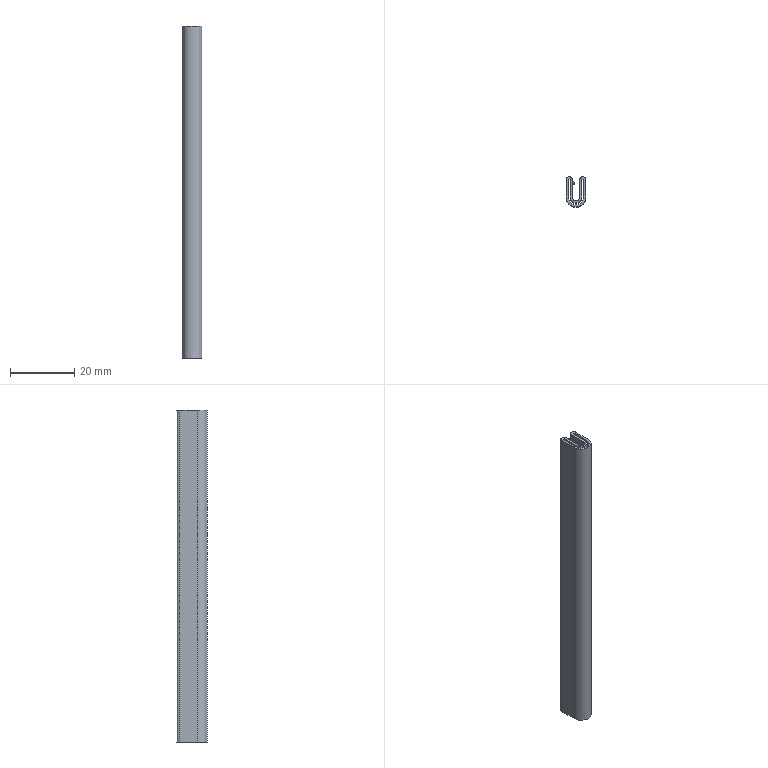Part | STEP file | TRAT2_4_B_3L1_TRAT2.4-B-3-L1 | 1 solid | 22 faces | box 6.2 x 9.5 x 103.6 mm | volume 2671 mm3 | plane 15 | cylinder 7 | commonest cylinder face diameters 1.9 x2 0.4 x1 2.4 x1 3.692 x1 4.933 x1 6.2 x1
STEP:
#1=CARTESIAN_POINT('',(1.9,8.55,103.6));
#2=VERTEX_POINT('',#1);
#3=CARTESIAN_POINT('',(0.,8.55,103.6));
#4=VERTEX_POINT('',#3);
#5=CARTESIAN_POINT('',(0.95,8.55,103.6));
#6=DIRECTION('',(0.,0.,1.));
#7=DIRECTION('',(1.,0.,0.));
#8=AXIS2_PLACEMENT_3D('',#5,#6,#7);
#9=CIRCLE('',#8,0.95);
#10=EDGE_CURVE('',#2,#4,#9,.T.);
#11=ORIENTED_EDGE('',*,*,#10,.T.);
#12=CARTESIAN_POINT('',(0.,3.1,103.6));
#13=VERTEX_POINT('',#12);
#14=CARTESIAN_POINT('',(0.,8.55,103.6));
#15=DIRECTION('',(0.,-1.,0.));
#16=VECTOR('',#15,1000.);
#17=LINE('',#14,#16);
#18=EDGE_CURVE('',#4,#13,#17,.T.);
#19=ORIENTED_EDGE('',*,*,#18,.T.);
#20=CARTESIAN_POINT('',(6.2,3.1,103.6));
#21=VERTEX_POINT('',#20);
#22=CARTESIAN_POINT('',(3.1,3.1,103.6));
#23=DIRECTION('',(0.,0.,1.));
#24=DIRECTION('',(1.,0.,0.));
#25=AXIS2_PLACEMENT_3D('',#22,#23,#24);
#26=CIRCLE('',#25,3.1);
#27=EDGE_CURVE('',#13,#21,#26,.T.);
#28=ORIENTED_EDGE('',*,*,#27,.T.);
#29=CARTESIAN_POINT('',(6.2,8.55,103.6));
#30=VERTEX_POINT('',#29);
#31=CARTESIAN_POINT('',(6.2,3.1,103.6));
#32=DIRECTION('',(0.,1.,0.));
#33=VECTOR('',#32,1000.);
#34=LINE('',#31,#33);
#35=EDGE_CURVE('',#21,#30,#34,.T.);
#36=ORIENTED_EDGE('',*,*,#35,.T.);
#37=CARTESIAN_POINT('',(4.3,8.55,103.6));
#38=VERTEX_POINT('',#37);
#39=CARTESIAN_POINT('',(5.25,8.55,103.6));
#40=DIRECTION('',(0.,0.,1.));
#41=DIRECTION('',(1.,0.,0.));
#42=AXIS2_PLACEMENT_3D('',#39,#40,#41);
#43=CIRCLE('',#42,0.95);
#44=EDGE_CURVE('',#30,#38,#43,.T.);
#45=ORIENTED_EDGE('',*,*,#44,.T.);
#46=CARTESIAN_POINT('',(4.3,3.1,103.6));
#47=VERTEX_POINT('',#46);
#48=CARTESIAN_POINT('',(4.3,8.55,103.6));
#49=DIRECTION('',(0.,-1.,0.));
#50=VECTOR('',#49,1000.);
#51=LINE('',#48,#50);
#52=EDGE_CURVE('',#38,#47,#51,.T.);
#53=ORIENTED_EDGE('',*,*,#52,.T.);
#54=CARTESIAN_POINT('',(1.9,3.1,103.6));
#55=VERTEX_POINT('',#54);
#56=CARTESIAN_POINT('',(3.1,3.1,103.6));
#57=DIRECTION('',(0.,0.,-1.));
#58=DIRECTION('',(-1.,0.,0.));
#59=AXIS2_PLACEMENT_3D('',#56,#57,#58);
#60=CIRCLE('',#59,1.2);
#61=EDGE_CURVE('',#47,#55,#60,.T.);
#62=ORIENTED_EDGE('',*,*,#61,.T.);
#63=CARTESIAN_POINT('',(1.9,7.6,103.6));
#64=VERTEX_POINT('',#63);
#65=CARTESIAN_POINT('',(1.9,3.1,103.6));
#66=DIRECTION('',(0.,1.,0.));
#67=VECTOR('',#66,1000.);
#68=LINE('',#65,#67);
#69=EDGE_CURVE('',#55,#64,#68,.T.);
#70=ORIENTED_EDGE('',*,*,#69,.T.);
#71=CARTESIAN_POINT('',(2.472,7.27,103.6));
#72=VERTEX_POINT('',#71);
#73=CARTESIAN_POINT('',(1.9,7.6,103.6));
#74=DIRECTION('',(0.866,-0.5,0.));
#75=VECTOR('',#74,1000.);
#76=LINE('',#73,#75);
#77=EDGE_CURVE('',#64,#72,#76,.T.);
#78=ORIENTED_EDGE('',*,*,#77,.T.);
#79=CARTESIAN_POINT('',(2.672,7.616,103.6));
#80=VERTEX_POINT('',#79);
#81=CARTESIAN_POINT('',(2.572,7.443,103.6));
#82=DIRECTION('',(0.,0.,1.));
#83=DIRECTION('',(1.,0.,0.));
#84=AXIS2_PLACEMENT_3D('',#81,#82,#83);
#85=CIRCLE('',#84,0.2);
#86=EDGE_CURVE('',#72,#80,#85,.T.);
#87=ORIENTED_EDGE('',*,*,#86,.T.);
#88=CARTESIAN_POINT('',(1.9,8.062,103.6));
#89=VERTEX_POINT('',#88);
#90=CARTESIAN_POINT('',(2.672,7.616,103.6));
#91=DIRECTION('',(-0.866,0.5,0.));
#92=VECTOR('',#91,1000.);
#93=LINE('',#90,#92);
#94=EDGE_CURVE('',#80,#89,#93,.T.);
#95=ORIENTED_EDGE('',*,*,#94,.T.);
#96=CARTESIAN_POINT('',(1.9,8.062,103.6));
#97=DIRECTION('',(0.,1.,0.));
#98=VECTOR('',#97,1000.);
#99=LINE('',#96,#98);
#100=EDGE_CURVE('',#89,#2,#99,.T.);
#101=ORIENTED_EDGE('',*,*,#100,.T.);
#102=EDGE_LOOP('',(#11,#19,#28,#36,#45,#53,#62,#70,#78,#87,#95,#101));
#103=FACE_OUTER_BOUND('',#102,.T.);
#104=CARTESIAN_POINT('',(0.6333,8.55,103.6));
#105=VERTEX_POINT('',#104);
#106=CARTESIAN_POINT('',(0.6333,3.1,103.6));
#107=VERTEX_POINT('',#106);
#108=CARTESIAN_POINT('',(0.6333,8.55,103.6));
#109=DIRECTION('',(0.,-1.,0.));
#110=VECTOR('',#109,1000.);
#111=LINE('',#108,#110);
#112=EDGE_CURVE('',#105,#107,#111,.T.);
#113=ORIENTED_EDGE('',*,*,#112,.F.);
#114=CARTESIAN_POINT('',(1.254,8.55,103.6));
#115=VERTEX_POINT('',#114);
#116=CARTESIAN_POINT('',(1.254,8.55,103.6));
#117=DIRECTION('',(-1.,0.,0.));
#118=VECTOR('',#117,1000.);
#119=LINE('',#116,#118);
#120=EDGE_CURVE('',#115,#105,#119,.T.);
#121=ORIENTED_EDGE('',*,*,#120,.F.);
#122=CARTESIAN_POINT('',(1.254,3.1,103.6));
#123=VERTEX_POINT('',#122);
#124=CARTESIAN_POINT('',(1.254,3.1,103.6));
#125=DIRECTION('',(0.,1.,0.));
#126=VECTOR('',#125,1000.);
#127=LINE('',#124,#126);
#128=EDGE_CURVE('',#123,#115,#127,.T.);
#129=ORIENTED_EDGE('',*,*,#128,.F.);
#130=CARTESIAN_POINT('',(4.946,3.1,103.6));
#131=VERTEX_POINT('',#130);
#132=CARTESIAN_POINT('',(3.1,3.1,103.6));
#133=DIRECTION('',(0.,0.,-1.));
#134=DIRECTION('',(-1.,0.,0.));
#135=AXIS2_PLACEMENT_3D('',#132,#133,#134);
#136=CIRCLE('',#135,1.846);
#137=EDGE_CURVE('',#131,#123,#136,.T.);
#138=ORIENTED_EDGE('',*,*,#137,.F.);
#139=CARTESIAN_POINT('',(4.946,8.55,103.6));
#140=VERTEX_POINT('',#139);
#141=CARTESIAN_POINT('',(4.946,8.55,103.6));
#142=DIRECTION('',(0.,-1.,0.));
#143=VECTOR('',#142,1000.);
#144=LINE('',#141,#143);
#145=EDGE_CURVE('',#140,#131,#144,.T.);
#146=ORIENTED_EDGE('',*,*,#145,.F.);
#147=CARTESIAN_POINT('',(5.567,8.55,103.6));
#148=VERTEX_POINT('',#147);
#149=CARTESIAN_POINT('',(5.567,8.55,103.6));
#150=DIRECTION('',(-1.,0.,0.));
#151=VECTOR('',#150,1000.);
#152=LINE('',#149,#151);
#153=EDGE_CURVE('',#148,#140,#152,.T.);
#154=ORIENTED_EDGE('',*,*,#153,.F.);
#155=CARTESIAN_POINT('',(5.567,3.1,103.6));
#156=VERTEX_POINT('',#155);
#157=CARTESIAN_POINT('',(5.567,3.1,103.6));
#158=DIRECTION('',(0.,1.,0.));
#159=VECTOR('',#158,1000.);
#160=LINE('',#157,#159);
#161=EDGE_CURVE('',#156,#148,#160,.T.);
#162=ORIENTED_EDGE('',*,*,#161,.F.);
#163=CARTESIAN_POINT('',(3.1,3.1,103.6));
#164=DIRECTION('',(0.,0.,1.));
#165=DIRECTION('',(1.,0.,0.));
#166=AXIS2_PLACEMENT_3D('',#163,#164,#165);
#167=CIRCLE('',#166,2.467);
#168=EDGE_CURVE('',#107,#156,#167,.T.);
#169=ORIENTED_EDGE('',*,*,#168,.F.);
#170=EDGE_LOOP('',(#113,#121,#129,#138,#146,#154,#162,#169));
#171=FACE_BOUND('',#170,.T.);
#172=CARTESIAN_POINT('',(0.95,8.55,103.6));
#173=DIRECTION('',(0.,0.,1.));
#174=DIRECTION('',(1.,0.,0.));
#175=AXIS2_PLACEMENT_3D('',#172,#173,#174);
#176=PLANE('',#175);
#177=ADVANCED_FACE('',(#103,#171),#176,.T.);
#178=CARTESIAN_POINT('',(1.9,8.55,0.));
#179=VERTEX_POINT('',#178);
#180=CARTESIAN_POINT('',(0.,8.55,0.));
#181=VERTEX_POINT('',#180);
#182=CARTESIAN_POINT('',(0.95,8.55,0.));
#183=DIRECTION('',(0.,0.,1.));
#184=DIRECTION('',(1.,0.,0.));
#185=AXIS2_PLACEMENT_3D('',#182,#183,#184);
#186=CIRCLE('',#185,0.95);
#187=EDGE_CURVE('',#179,#181,#186,.T.);
#188=ORIENTED_EDGE('',*,*,#187,.F.);
#189=CARTESIAN_POINT('',(1.9,8.062,0.));
#190=VERTEX_POINT('',#189);
#191=CARTESIAN_POINT('',(1.9,8.062,0.));
#192=DIRECTION('',(0.,1.,0.));
#193=VECTOR('',#192,1000.);
#194=LINE('',#191,#193);
#195=EDGE_CURVE('',#190,#179,#194,.T.);
#196=ORIENTED_EDGE('',*,*,#195,.F.);
#197=CARTESIAN_POINT('',(2.672,7.616,0.));
#198=VERTEX_POINT('',#197);
#199=CARTESIAN_POINT('',(2.672,7.616,0.));
#200=DIRECTION('',(-0.866,0.5,0.));
#201=VECTOR('',#200,1000.);
#202=LINE('',#199,#201);
#203=EDGE_CURVE('',#198,#190,#202,.T.);
#204=ORIENTED_EDGE('',*,*,#203,.F.);
#205=CARTESIAN_POINT('',(2.472,7.27,0.));
#206=VERTEX_POINT('',#205);
#207=CARTESIAN_POINT('',(2.572,7.443,0.));
#208=DIRECTION('',(0.,0.,1.));
#209=DIRECTION('',(1.,0.,0.));
#210=AXIS2_PLACEMENT_3D('',#207,#208,#209);
#211=CIRCLE('',#210,0.2);
#212=EDGE_CURVE('',#206,#198,#211,.T.);
#213=ORIENTED_EDGE('',*,*,#212,.F.);
#214=CARTESIAN_POINT('',(1.9,7.6,0.));
#215=VERTEX_POINT('',#214);
#216=CARTESIAN_POINT('',(1.9,7.6,0.));
#217=DIRECTION('',(0.866,-0.5,0.));
#218=VECTOR('',#217,1000.);
#219=LINE('',#216,#218);
#220=EDGE_CURVE('',#215,#206,#219,.T.);
#221=ORIENTED_EDGE('',*,*,#220,.F.);
#222=CARTESIAN_POINT('',(1.9,3.1,0.));
#223=VERTEX_POINT('',#222);
#224=CARTESIAN_POINT('',(1.9,3.1,0.));
#225=DIRECTION('',(0.,1.,0.));
#226=VECTOR('',#225,1000.);
#227=LINE('',#224,#226);
#228=EDGE_CURVE('',#223,#215,#227,.T.);
#229=ORIENTED_EDGE('',*,*,#228,.F.);
#230=CARTESIAN_POINT('',(4.3,3.1,0.));
#231=VERTEX_POINT('',#230);
#232=CARTESIAN_POINT('',(3.1,3.1,0.));
#233=DIRECTION('',(0.,0.,-1.));
#234=DIRECTION('',(-1.,0.,0.));
#235=AXIS2_PLACEMENT_3D('',#232,#233,#234);
#236=CIRCLE('',#235,1.2);
#237=EDGE_CURVE('',#231,#223,#236,.T.);
#238=ORIENTED_EDGE('',*,*,#237,.F.);
#239=CARTESIAN_POINT('',(4.3,8.55,0.));
#240=VERTEX_POINT('',#239);
#241=CARTESIAN_POINT('',(4.3,8.55,0.));
#242=DIRECTION('',(0.,-1.,0.));
#243=VECTOR('',#242,1000.);
#244=LINE('',#241,#243);
#245=EDGE_CURVE('',#240,#231,#244,.T.);
#246=ORIENTED_EDGE('',*,*,#245,.F.);
#247=CARTESIAN_POINT('',(6.2,8.55,0.));
#248=VERTEX_POINT('',#247);
#249=CARTESIAN_POINT('',(5.25,8.55,0.));
#250=DIRECTION('',(0.,0.,1.));
#251=DIRECTION('',(1.,0.,0.));
#252=AXIS2_PLACEMENT_3D('',#249,#250,#251);
#253=CIRCLE('',#252,0.95);
#254=EDGE_CURVE('',#248,#240,#253,.T.);
#255=ORIENTED_EDGE('',*,*,#254,.F.);
#256=CARTESIAN_POINT('',(6.2,3.1,0.));
#257=VERTEX_POINT('',#256);
#258=CARTESIAN_POINT('',(6.2,3.1,0.));
#259=DIRECTION('',(0.,1.,0.));
#260=VECTOR('',#259,1000.);
#261=LINE('',#258,#260);
#262=EDGE_CURVE('',#257,#248,#261,.T.);
#263=ORIENTED_EDGE('',*,*,#262,.F.);
#264=CARTESIAN_POINT('',(0.,3.1,0.));
#265=VERTEX_POINT('',#264);
#266=CARTESIAN_POINT('',(3.1,3.1,0.));
#267=DIRECTION('',(0.,0.,1.));
#268=DIRECTION('',(1.,0.,0.));
#269=AXIS2_PLACEMENT_3D('',#266,#267,#268);
#270=CIRCLE('',#269,3.1);
#271=EDGE_CURVE('',#265,#257,#270,.T.);
#272=ORIENTED_EDGE('',*,*,#271,.F.);
#273=CARTESIAN_POINT('',(0.,8.55,0.));
#274=DIRECTION('',(0.,-1.,0.));
#275=VECTOR('',#274,1000.);
#276=LINE('',#273,#275);
#277=EDGE_CURVE('',#181,#265,#276,.T.);
#278=ORIENTED_EDGE('',*,*,#277,.F.);
#279=EDGE_LOOP('',(#188,#196,#204,#213,#221,#229,#238,#246,#255,#263,#272,#278));
#280=FACE_OUTER_BOUND('',#279,.T.);
#281=CARTESIAN_POINT('',(1.254,8.55,0.));
#282=VERTEX_POINT('',#281);
#283=CARTESIAN_POINT('',(0.6333,8.55,0.));
#284=VERTEX_POINT('',#283);
#285=CARTESIAN_POINT('',(1.254,8.55,0.));
#286=DIRECTION('',(-1.,0.,0.));
#287=VECTOR('',#286,1000.);
#288=LINE('',#285,#287);
#289=EDGE_CURVE('',#282,#284,#288,.T.);
#290=ORIENTED_EDGE('',*,*,#289,.T.);
#291=CARTESIAN_POINT('',(0.6333,3.1,0.));
#292=VERTEX_POINT('',#291);
#293=CARTESIAN_POINT('',(0.6333,8.55,0.));
#294=DIRECTION('',(0.,-1.,0.));
#295=VECTOR('',#294,1000.);
#296=LINE('',#293,#295);
#297=EDGE_CURVE('',#284,#292,#296,.T.);
#298=ORIENTED_EDGE('',*,*,#297,.T.);
#299=CARTESIAN_POINT('',(5.567,3.1,0.));
#300=VERTEX_POINT('',#299);
#301=CARTESIAN_POINT('',(3.1,3.1,0.));
#302=DIRECTION('',(0.,0.,1.));
#303=DIRECTION('',(1.,0.,0.));
#304=AXIS2_PLACEMENT_3D('',#301,#302,#303);
#305=CIRCLE('',#304,2.467);
#306=EDGE_CURVE('',#292,#300,#305,.T.);
#307=ORIENTED_EDGE('',*,*,#306,.T.);
#308=CARTESIAN_POINT('',(5.567,8.55,0.));
#309=VERTEX_POINT('',#308);
#310=CARTESIAN_POINT('',(5.567,3.1,0.));
#311=DIRECTION('',(0.,1.,0.));
#312=VECTOR('',#311,1000.);
#313=LINE('',#310,#312);
#314=EDGE_CURVE('',#300,#309,#313,.T.);
#315=ORIENTED_EDGE('',*,*,#314,.T.);
#316=CARTESIAN_POINT('',(4.946,8.55,0.));
#317=VERTEX_POINT('',#316);
#318=CARTESIAN_POINT('',(5.567,8.55,0.));
#319=DIRECTION('',(-1.,0.,0.));
#320=VECTOR('',#319,1000.);
#321=LINE('',#318,#320);
#322=EDGE_CURVE('',#309,#317,#321,.T.);
#323=ORIENTED_EDGE('',*,*,#322,.T.);
#324=CARTESIAN_POINT('',(4.946,3.1,0.));
#325=VERTEX_POINT('',#324);
#326=CARTESIAN_POINT('',(4.946,8.55,0.));
#327=DIRECTION('',(0.,-1.,0.));
#328=VECTOR('',#327,1000.);
#329=LINE('',#326,#328);
#330=EDGE_CURVE('',#317,#325,#329,.T.);
#331=ORIENTED_EDGE('',*,*,#330,.T.);
#332=CARTESIAN_POINT('',(1.254,3.1,0.));
#333=VERTEX_POINT('',#332);
#334=CARTESIAN_POINT('',(3.1,3.1,0.));
#335=DIRECTION('',(0.,0.,-1.));
#336=DIRECTION('',(-1.,0.,0.));
#337=AXIS2_PLACEMENT_3D('',#334,#335,#336);
#338=CIRCLE('',#337,1.846);
#339=EDGE_CURVE('',#325,#333,#338,.T.);
#340=ORIENTED_EDGE('',*,*,#339,.T.);
#341=CARTESIAN_POINT('',(1.254,3.1,0.));
#342=DIRECTION('',(0.,1.,0.));
#343=VECTOR('',#342,1000.);
#344=LINE('',#341,#343);
#345=EDGE_CURVE('',#333,#282,#344,.T.);
#346=ORIENTED_EDGE('',*,*,#345,.T.);
#347=EDGE_LOOP('',(#290,#298,#307,#315,#323,#331,#340,#346));
#348=FACE_BOUND('',#347,.T.);
#349=CARTESIAN_POINT('',(0.95,8.55,0.));
#350=DIRECTION('',(0.,0.,1.));
#351=DIRECTION('',(1.,0.,0.));
#352=AXIS2_PLACEMENT_3D('',#349,#350,#351);
#353=PLANE('',#352);
#354=ADVANCED_FACE('',(#280,#348),#353,.F.);
#355=ORIENTED_EDGE('',*,*,#187,.T.);
#356=CARTESIAN_POINT('',(0.,8.55,103.6));
#357=DIRECTION('',(0.,0.,-1.));
#358=VECTOR('',#357,1000.);
#359=LINE('',#356,#358);
#360=EDGE_CURVE('',#4,#181,#359,.T.);
#361=ORIENTED_EDGE('',*,*,#360,.F.);
#362=ORIENTED_EDGE('',*,*,#10,.F.);
#363=CARTESIAN_POINT('',(1.9,8.55,103.6));
#364=DIRECTION('',(0.,0.,-1.));
#365=VECTOR('',#364,1000.);
#366=LINE('',#363,#365);
#367=EDGE_CURVE('',#2,#179,#366,.T.);
#368=ORIENTED_EDGE('',*,*,#367,.T.);
#369=EDGE_LOOP('',(#355,#361,#362,#368));
#370=FACE_OUTER_BOUND('',#369,.T.);
#371=CARTESIAN_POINT('',(0.95,8.55,103.6));
#372=DIRECTION('',(0.,0.,-1.));
#373=DIRECTION('',(-1.,0.,0.));
#374=AXIS2_PLACEMENT_3D('',#371,#372,#373);
#375=CYLINDRICAL_SURFACE('',#374,0.95);
#376=ADVANCED_FACE('',(#370),#375,.T.);
#377=ORIENTED_EDGE('',*,*,#277,.T.);
#378=CARTESIAN_POINT('',(0.,3.1,103.6));
#379=DIRECTION('',(0.,0.,-1.));
#380=VECTOR('',#379,1000.);
#381=LINE('',#378,#380);
#382=EDGE_CURVE('',#13,#265,#381,.T.);
#383=ORIENTED_EDGE('',*,*,#382,.F.);
#384=ORIENTED_EDGE('',*,*,#18,.F.);
#385=ORIENTED_EDGE('',*,*,#360,.T.);
#386=EDGE_LOOP('',(#377,#383,#384,#385));
#387=FACE_OUTER_BOUND('',#386,.T.);
#388=CARTESIAN_POINT('',(0.,8.55,103.6));
#389=DIRECTION('',(1.,0.,0.));
#390=DIRECTION('',(0.,0.,-1.));
#391=AXIS2_PLACEMENT_3D('',#388,#389,#390);
#392=PLANE('',#391);
#393=ADVANCED_FACE('',(#387),#392,.F.);
#394=ORIENTED_EDGE('',*,*,#271,.T.);
#395=CARTESIAN_POINT('',(6.2,3.1,103.6));
#396=DIRECTION('',(0.,0.,-1.));
#397=VECTOR('',#396,1000.);
#398=LINE('',#395,#397);
#399=EDGE_CURVE('',#21,#257,#398,.T.);
#400=ORIENTED_EDGE('',*,*,#399,.F.);
#401=ORIENTED_EDGE('',*,*,#27,.F.);
#402=ORIENTED_EDGE('',*,*,#382,.T.);
#403=EDGE_LOOP('',(#394,#400,#401,#402));
#404=FACE_OUTER_BOUND('',#403,.T.);
#405=CARTESIAN_POINT('',(3.1,3.1,103.6));
#406=DIRECTION('',(0.,0.,-1.));
#407=DIRECTION('',(-1.,0.,0.));
#408=AXIS2_PLACEMENT_3D('',#405,#406,#407);
#409=CYLINDRICAL_SURFACE('',#408,3.1);
#410=ADVANCED_FACE('',(#404),#409,.T.);
#411=ORIENTED_EDGE('',*,*,#262,.T.);
#412=CARTESIAN_POINT('',(6.2,8.55,103.6));
#413=DIRECTION('',(0.,0.,-1.));
#414=VECTOR('',#413,1000.);
#415=LINE('',#412,#414);
#416=EDGE_CURVE('',#30,#248,#415,.T.);
#417=ORIENTED_EDGE('',*,*,#416,.F.);
#418=ORIENTED_EDGE('',*,*,#35,.F.);
#419=ORIENTED_EDGE('',*,*,#399,.T.);
#420=EDGE_LOOP('',(#411,#417,#418,#419));
#421=FACE_OUTER_BOUND('',#420,.T.);
#422=CARTESIAN_POINT('',(6.2,3.1,103.6));
#423=DIRECTION('',(-1.,0.,0.));
#424=DIRECTION('',(0.,0.,1.));
#425=AXIS2_PLACEMENT_3D('',#422,#423,#424);
#426=PLANE('',#425);
#427=ADVANCED_FACE('',(#421),#426,.F.);
#428=ORIENTED_EDGE('',*,*,#254,.T.);
#429=CARTESIAN_POINT('',(4.3,8.55,103.6));
#430=DIRECTION('',(0.,0.,-1.));
#431=VECTOR('',#430,1000.);
#432=LINE('',#429,#431);
#433=EDGE_CURVE('',#38,#240,#432,.T.);
#434=ORIENTED_EDGE('',*,*,#433,.F.);
#435=ORIENTED_EDGE('',*,*,#44,.F.);
#436=ORIENTED_EDGE('',*,*,#416,.T.);
#437=EDGE_LOOP('',(#428,#434,#435,#436));
#438=FACE_OUTER_BOUND('',#437,.T.);
#439=CARTESIAN_POINT('',(5.25,8.55,103.6));
#440=DIRECTION('',(0.,0.,-1.));
#441=DIRECTION('',(-1.,0.,0.));
#442=AXIS2_PLACEMENT_3D('',#439,#440,#441);
#443=CYLINDRICAL_SURFACE('',#442,0.95);
#444=ADVANCED_FACE('',(#438),#443,.T.);
#445=ORIENTED_EDGE('',*,*,#245,.T.);
#446=CARTESIAN_POINT('',(4.3,3.1,103.6));
#447=DIRECTION('',(0.,0.,-1.));
#448=VECTOR('',#447,1000.);
#449=LINE('',#446,#448);
#450=EDGE_CURVE('',#47,#231,#449,.T.);
#451=ORIENTED_EDGE('',*,*,#450,.F.);
#452=ORIENTED_EDGE('',*,*,#52,.F.);
#453=ORIENTED_EDGE('',*,*,#433,.T.);
#454=EDGE_LOOP('',(#445,#451,#452,#453));
#455=FACE_OUTER_BOUND('',#454,.T.);
#456=CARTESIAN_POINT('',(4.3,8.55,103.6));
#457=DIRECTION('',(1.,0.,0.));
#458=DIRECTION('',(0.,1.,0.));
#459=AXIS2_PLACEMENT_3D('',#456,#457,#458);
#460=PLANE('',#459);
#461=ADVANCED_FACE('',(#455),#460,.F.);
#462=ORIENTED_EDGE('',*,*,#237,.T.);
#463=CARTESIAN_POINT('',(1.9,3.1,103.6));
#464=DIRECTION('',(0.,0.,-1.));
#465=VECTOR('',#464,1000.);
#466=LINE('',#463,#465);
#467=EDGE_CURVE('',#55,#223,#466,.T.);
#468=ORIENTED_EDGE('',*,*,#467,.F.);
#469=ORIENTED_EDGE('',*,*,#61,.F.);
#470=ORIENTED_EDGE('',*,*,#450,.T.);
#471=EDGE_LOOP('',(#462,#468,#469,#470));
#472=FACE_OUTER_BOUND('',#471,.T.);
#473=CARTESIAN_POINT('',(3.1,3.1,103.6));
#474=DIRECTION('',(0.,0.,-1.));
#475=DIRECTION('',(-1.,0.,0.));
#476=AXIS2_PLACEMENT_3D('',#473,#474,#475);
#477=CYLINDRICAL_SURFACE('',#476,1.2);
#478=ADVANCED_FACE('',(#472),#477,.F.);
#479=ORIENTED_EDGE('',*,*,#228,.T.);
#480=CARTESIAN_POINT('',(1.9,7.6,103.6));
#481=DIRECTION('',(0.,0.,-1.));
#482=VECTOR('',#481,1000.);
#483=LINE('',#480,#482);
#484=EDGE_CURVE('',#64,#215,#483,.T.);
#485=ORIENTED_EDGE('',*,*,#484,.F.);
#486=ORIENTED_EDGE('',*,*,#69,.F.);
#487=ORIENTED_EDGE('',*,*,#467,.T.);
#488=EDGE_LOOP('',(#479,#485,#486,#487));
#489=FACE_OUTER_BOUND('',#488,.T.);
#490=CARTESIAN_POINT('',(1.9,3.1,103.6));
#491=DIRECTION('',(-1.,0.,0.));
#492=DIRECTION('',(0.,-1.,0.));
#493=AXIS2_PLACEMENT_3D('',#490,#491,#492);
#494=PLANE('',#493);
#495=ADVANCED_FACE('',(#489),#494,.F.);
#496=ORIENTED_EDGE('',*,*,#220,.T.);
#497=CARTESIAN_POINT('',(2.472,7.27,103.6));
#498=DIRECTION('',(0.,0.,-1.));
#499=VECTOR('',#498,1000.);
#500=LINE('',#497,#499);
#501=EDGE_CURVE('',#72,#206,#500,.T.);
#502=ORIENTED_EDGE('',*,*,#501,.F.);
#503=ORIENTED_EDGE('',*,*,#77,.F.);
#504=ORIENTED_EDGE('',*,*,#484,.T.);
#505=EDGE_LOOP('',(#496,#502,#503,#504));
#506=FACE_OUTER_BOUND('',#505,.T.);
#507=CARTESIAN_POINT('',(1.9,7.6,103.6));
#508=DIRECTION('',(0.5,0.866,0.));
#509=DIRECTION('',(-0.866,0.5,0.));
#510=AXIS2_PLACEMENT_3D('',#507,#508,#509);
#511=PLANE('',#510);
#512=ADVANCED_FACE('',(#506),#511,.F.);
#513=ORIENTED_EDGE('',*,*,#212,.T.);
#514=CARTESIAN_POINT('',(2.672,7.616,103.6));
#515=DIRECTION('',(0.,0.,-1.));
#516=VECTOR('',#515,1000.);
#517=LINE('',#514,#516);
#518=EDGE_CURVE('',#80,#198,#517,.T.);
#519=ORIENTED_EDGE('',*,*,#518,.F.);
#520=ORIENTED_EDGE('',*,*,#86,.F.);
#521=ORIENTED_EDGE('',*,*,#501,.T.);
#522=EDGE_LOOP('',(#513,#519,#520,#521));
#523=FACE_OUTER_BOUND('',#522,.T.);
#524=CARTESIAN_POINT('',(2.572,7.443,103.6));
#525=DIRECTION('',(0.,0.,-1.));
#526=DIRECTION('',(-1.,0.,0.));
#527=AXIS2_PLACEMENT_3D('',#524,#525,#526);
#528=CYLINDRICAL_SURFACE('',#527,0.2);
#529=ADVANCED_FACE('',(#523),#528,.T.);
#530=ORIENTED_EDGE('',*,*,#203,.T.);
#531=CARTESIAN_POINT('',(1.9,8.062,103.6));
#532=DIRECTION('',(0.,0.,-1.));
#533=VECTOR('',#532,1000.);
#534=LINE('',#531,#533);
#535=EDGE_CURVE('',#89,#190,#534,.T.);
#536=ORIENTED_EDGE('',*,*,#535,.F.);
#537=ORIENTED_EDGE('',*,*,#94,.F.);
#538=ORIENTED_EDGE('',*,*,#518,.T.);
#539=EDGE_LOOP('',(#530,#536,#537,#538));
#540=FACE_OUTER_BOUND('',#539,.T.);
#541=CARTESIAN_POINT('',(2.672,7.616,103.6));
#542=DIRECTION('',(-0.5,-0.866,0.));
#543=DIRECTION('',(0.866,-0.5,0.));
#544=AXIS2_PLACEMENT_3D('',#541,#542,#543);
#545=PLANE('',#544);
#546=ADVANCED_FACE('',(#540),#545,.F.);
#547=ORIENTED_EDGE('',*,*,#195,.T.);
#548=ORIENTED_EDGE('',*,*,#367,.F.);
#549=ORIENTED_EDGE('',*,*,#100,.F.);
#550=ORIENTED_EDGE('',*,*,#535,.T.);
#551=EDGE_LOOP('',(#547,#548,#549,#550));
#552=FACE_OUTER_BOUND('',#551,.T.);
#553=CARTESIAN_POINT('',(1.9,8.062,103.6));
#554=DIRECTION('',(-1.,0.,0.));
#555=DIRECTION('',(0.,0.,1.));
#556=AXIS2_PLACEMENT_3D('',#553,#554,#555);
#557=PLANE('',#556);
#558=ADVANCED_FACE('',(#552),#557,.F.);
#559=ORIENTED_EDGE('',*,*,#289,.F.);
#560=CARTESIAN_POINT('',(1.254,8.55,103.6));
#561=DIRECTION('',(0.,0.,-1.));
#562=VECTOR('',#561,1000.);
#563=LINE('',#560,#562);
#564=EDGE_CURVE('',#115,#282,#563,.T.);
#565=ORIENTED_EDGE('',*,*,#564,.F.);
#566=ORIENTED_EDGE('',*,*,#120,.T.);
#567=CARTESIAN_POINT('',(0.6333,8.55,103.6));
#568=DIRECTION('',(0.,0.,-1.));
#569=VECTOR('',#568,1000.);
#570=LINE('',#567,#569);
#571=EDGE_CURVE('',#105,#284,#570,.T.);
#572=ORIENTED_EDGE('',*,*,#571,.T.);
#573=EDGE_LOOP('',(#559,#565,#566,#572));
#574=FACE_OUTER_BOUND('',#573,.T.);
#575=CARTESIAN_POINT('',(1.254,8.55,103.6));
#576=DIRECTION('',(0.,-1.,0.));
#577=DIRECTION('',(0.,0.,-1.));
#578=AXIS2_PLACEMENT_3D('',#575,#576,#577);
#579=PLANE('',#578);
#580=ADVANCED_FACE('',(#574),#579,.T.);
#581=ORIENTED_EDGE('',*,*,#297,.F.);
#582=ORIENTED_EDGE('',*,*,#571,.F.);
#583=ORIENTED_EDGE('',*,*,#112,.T.);
#584=CARTESIAN_POINT('',(0.6333,3.1,103.6));
#585=DIRECTION('',(0.,0.,-1.));
#586=VECTOR('',#585,1000.);
#587=LINE('',#584,#586);
#588=EDGE_CURVE('',#107,#292,#587,.T.);
#589=ORIENTED_EDGE('',*,*,#588,.T.);
#590=EDGE_LOOP('',(#581,#582,#583,#589));
#591=FACE_OUTER_BOUND('',#590,.T.);
#592=CARTESIAN_POINT('',(0.6333,8.55,103.6));
#593=DIRECTION('',(1.,0.,0.));
#594=DIRECTION('',(0.,1.,0.));
#595=AXIS2_PLACEMENT_3D('',#592,#593,#594);
#596=PLANE('',#595);
#597=ADVANCED_FACE('',(#591),#596,.T.);
#598=ORIENTED_EDGE('',*,*,#306,.F.);
#599=ORIENTED_EDGE('',*,*,#588,.F.);
#600=ORIENTED_EDGE('',*,*,#168,.T.);
#601=CARTESIAN_POINT('',(5.567,3.1,103.6));
#602=DIRECTION('',(0.,0.,-1.));
#603=VECTOR('',#602,1000.);
#604=LINE('',#601,#603);
#605=EDGE_CURVE('',#156,#300,#604,.T.);
#606=ORIENTED_EDGE('',*,*,#605,.T.);
#607=EDGE_LOOP('',(#598,#599,#600,#606));
#608=FACE_OUTER_BOUND('',#607,.T.);
#609=CARTESIAN_POINT('',(3.1,3.1,103.6));
#610=DIRECTION('',(0.,0.,-1.));
#611=DIRECTION('',(-1.,0.,0.));
#612=AXIS2_PLACEMENT_3D('',#609,#610,#611);
#613=CYLINDRICAL_SURFACE('',#612,2.467);
#614=ADVANCED_FACE('',(#608),#613,.F.);
#615=ORIENTED_EDGE('',*,*,#314,.F.);
#616=ORIENTED_EDGE('',*,*,#605,.F.);
#617=ORIENTED_EDGE('',*,*,#161,.T.);
#618=CARTESIAN_POINT('',(5.567,8.55,103.6));
#619=DIRECTION('',(0.,0.,-1.));
#620=VECTOR('',#619,1000.);
#621=LINE('',#618,#620);
#622=EDGE_CURVE('',#148,#309,#621,.T.);
#623=ORIENTED_EDGE('',*,*,#622,.T.);
#624=EDGE_LOOP('',(#615,#616,#617,#623));
#625=FACE_OUTER_BOUND('',#624,.T.);
#626=CARTESIAN_POINT('',(5.567,3.1,103.6));
#627=DIRECTION('',(-1.,0.,0.));
#628=DIRECTION('',(0.,-1.,0.));
#629=AXIS2_PLACEMENT_3D('',#626,#627,#628);
#630=PLANE('',#629);
#631=ADVANCED_FACE('',(#625),#630,.T.);
#632=ORIENTED_EDGE('',*,*,#322,.F.);
#633=ORIENTED_EDGE('',*,*,#622,.F.);
#634=ORIENTED_EDGE('',*,*,#153,.T.);
#635=CARTESIAN_POINT('',(4.946,8.55,103.6));
#636=DIRECTION('',(0.,0.,-1.));
#637=VECTOR('',#636,1000.);
#638=LINE('',#635,#637);
#639=EDGE_CURVE('',#140,#317,#638,.T.);
#640=ORIENTED_EDGE('',*,*,#639,.T.);
#641=EDGE_LOOP('',(#632,#633,#634,#640));
#642=FACE_OUTER_BOUND('',#641,.T.);
#643=CARTESIAN_POINT('',(5.567,8.55,103.6));
#644=DIRECTION('',(0.,-1.,0.));
#645=DIRECTION('',(0.,0.,-1.));
#646=AXIS2_PLACEMENT_3D('',#643,#644,#645);
#647=PLANE('',#646);
#648=ADVANCED_FACE('',(#642),#647,.T.);
#649=ORIENTED_EDGE('',*,*,#330,.F.);
#650=ORIENTED_EDGE('',*,*,#639,.F.);
#651=ORIENTED_EDGE('',*,*,#145,.T.);
#652=CARTESIAN_POINT('',(4.946,3.1,103.6));
#653=DIRECTION('',(0.,0.,-1.));
#654=VECTOR('',#653,1000.);
#655=LINE('',#652,#654);
#656=EDGE_CURVE('',#131,#325,#655,.T.);
#657=ORIENTED_EDGE('',*,*,#656,.T.);
#658=EDGE_LOOP('',(#649,#650,#651,#657));
#659=FACE_OUTER_BOUND('',#658,.T.);
#660=CARTESIAN_POINT('',(4.946,8.55,103.6));
#661=DIRECTION('',(1.,0.,0.));
#662=DIRECTION('',(0.,0.,-1.));
#663=AXIS2_PLACEMENT_3D('',#660,#661,#662);
#664=PLANE('',#663);
#665=ADVANCED_FACE('',(#659),#664,.T.);
#666=ORIENTED_EDGE('',*,*,#339,.F.);
#667=ORIENTED_EDGE('',*,*,#656,.F.);
#668=ORIENTED_EDGE('',*,*,#137,.T.);
#669=CARTESIAN_POINT('',(1.254,3.1,103.6));
#670=DIRECTION('',(0.,0.,-1.));
#671=VECTOR('',#670,1000.);
#672=LINE('',#669,#671);
#673=EDGE_CURVE('',#123,#333,#672,.T.);
#674=ORIENTED_EDGE('',*,*,#673,.T.);
#675=EDGE_LOOP('',(#666,#667,#668,#674));
#676=FACE_OUTER_BOUND('',#675,.T.);
#677=CARTESIAN_POINT('',(3.1,3.1,103.6));
#678=DIRECTION('',(0.,0.,-1.));
#679=DIRECTION('',(-1.,0.,0.));
#680=AXIS2_PLACEMENT_3D('',#677,#678,#679);
#681=CYLINDRICAL_SURFACE('',#680,1.846);
#682=ADVANCED_FACE('',(#676),#681,.T.);
#683=ORIENTED_EDGE('',*,*,#345,.F.);
#684=ORIENTED_EDGE('',*,*,#673,.F.);
#685=ORIENTED_EDGE('',*,*,#128,.T.);
#686=ORIENTED_EDGE('',*,*,#564,.T.);
#687=EDGE_LOOP('',(#683,#684,#685,#686));
#688=FACE_OUTER_BOUND('',#687,.T.);
#689=CARTESIAN_POINT('',(1.254,3.1,103.6));
#690=DIRECTION('',(-1.,0.,0.));
#691=DIRECTION('',(0.,-1.,0.));
#692=AXIS2_PLACEMENT_3D('',#689,#690,#691);
#693=PLANE('',#692);
#694=ADVANCED_FACE('',(#688),#693,.T.);
#695=CLOSED_SHELL('',(#177,#354,#376,#393,#410,#427,#444,#461,#478,#495,#512,#529,#546,#558,#580,#597,#614,#631,#648,#665,#682,#694));
#696=MANIFOLD_SOLID_BREP('',#695);
#697=CARTESIAN_POINT('',(0.,0.,0.));
#698=DIRECTION('',(0.,0.,1.));
#699=DIRECTION('',(1.,0.,0.));
#700=AXIS2_PLACEMENT_3D('',#697,#698,#699);
#701=(LENGTH_UNIT()NAMED_UNIT(*)SI_UNIT(.MILLI.,.METRE.));
#702=UNCERTAINTY_MEASURE_WITH_UNIT(LENGTH_MEASURE(0.00001),#701,'','');
#703=(NAMED_UNIT(*)PLANE_ANGLE_UNIT()SI_UNIT($,.RADIAN.));
#704=(NAMED_UNIT(*)SI_UNIT($,.STERADIAN.)SOLID_ANGLE_UNIT());
#705=(GEOMETRIC_REPRESENTATION_CONTEXT(3)GLOBAL_UNCERTAINTY_ASSIGNED_CONTEXT((#702))GLOBAL_UNIT_ASSIGNED_CONTEXT((#701,#703,#704))REPRESENTATION_CONTEXT('',''));
#706=ADVANCED_BREP_SHAPE_REPRESENTATION('',(#696,#700),#705);